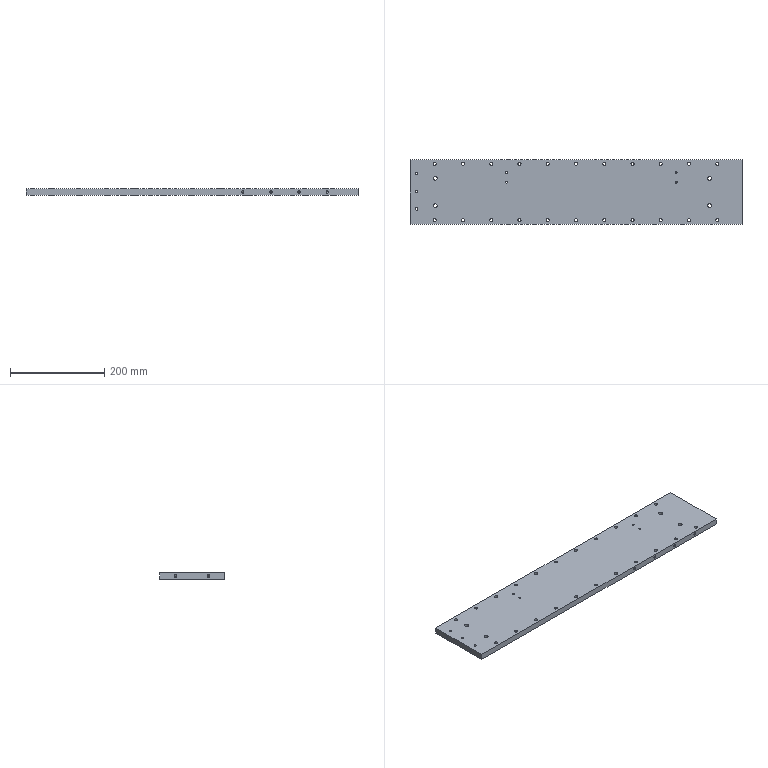Part | STEP file | PN_0085 crossbeam | 1 solid | 170 faces | box 705 x 138 x 13 mm | volume 1239081 mm3 | cylinder 126 | plane 28 | cone 16 | commonest cylinder face diameters 6.6 x44 11 x44 5 x22 4.2 x8 8.5 x8